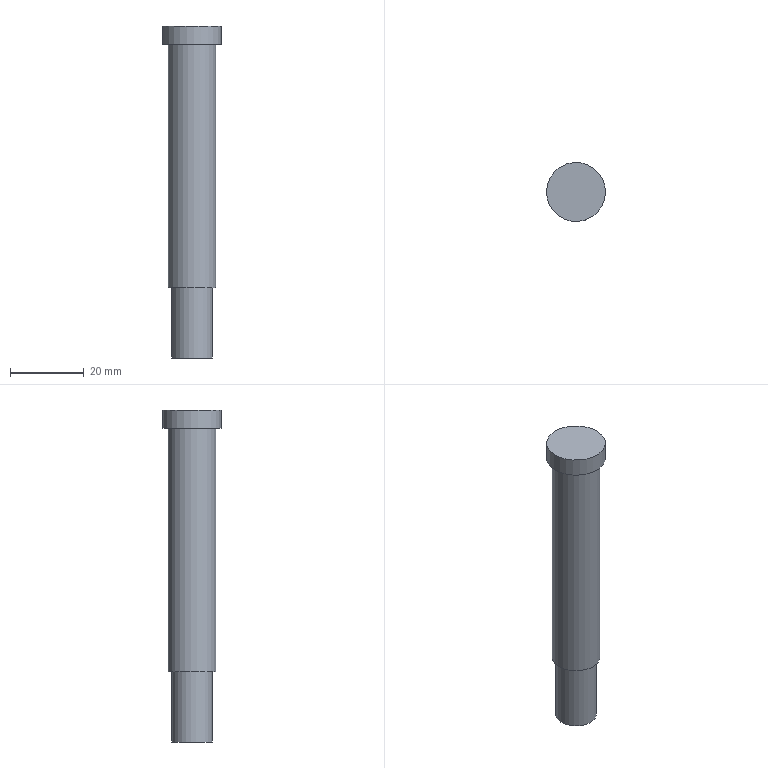Part | NX | features solid 2 | 1 solid | 7 faces | box 16 x 16 x 90 mm | volume 11604 mm3 | plane 4 | cylinder 3 | commonest cylinder face diameters 11.1 x1 13 x1 16 x1
STEP:
#1=CARTESIAN_POINT('',(-672.974,-368.75,22.));
#2=VERTEX_POINT('',#1);
#3=CARTESIAN_POINT('',(-678.603,-365.5,22.));
#4=DIRECTION('',(0.,0.,1.));
#5=DIRECTION('',(0.866,-0.5,0.));
#6=AXIS2_PLACEMENT_3D('',#3,#4,#5);
#7=CIRCLE('',#6,6.5);
#8=EDGE_CURVE('',#2,#2,#7,.T.);
#9=ORIENTED_EDGE('',*,*,#8,.T.);
#10=EDGE_LOOP('',(#9));
#11=FACE_BOUND('',#10,.T.);
#12=CARTESIAN_POINT('',(-672.974,-368.75,88.));
#13=VERTEX_POINT('',#12);
#14=CARTESIAN_POINT('',(-678.603,-365.5,88.));
#15=DIRECTION('',(0.,0.,1.));
#16=DIRECTION('',(0.866,-0.5,0.));
#17=AXIS2_PLACEMENT_3D('',#14,#15,#16);
#18=CIRCLE('',#17,6.5);
#19=EDGE_CURVE('',#13,#13,#18,.T.);
#20=ORIENTED_EDGE('',*,*,#19,.F.);
#21=EDGE_LOOP('',(#20));
#22=FACE_BOUND('',#21,.T.);
#23=CARTESIAN_POINT('',(-678.603,-365.5,93.));
#24=DIRECTION('',(0.,0.,-1.));
#25=DIRECTION('',(-0.866,0.5,0.));
#26=AXIS2_PLACEMENT_3D('',#23,#24,#25);
#27=CYLINDRICAL_SURFACE('',#26,6.5);
#28=ADVANCED_FACE('',(#11,#22),#27,.T.);
#29=CARTESIAN_POINT('',(-673.797,-368.275,22.));
#30=VERTEX_POINT('',#29);
#31=CARTESIAN_POINT('',(-678.603,-365.5,22.));
#32=DIRECTION('',(0.,0.,1.));
#33=DIRECTION('',(0.866,-0.5,0.));
#34=AXIS2_PLACEMENT_3D('',#31,#32,#33);
#35=CIRCLE('',#34,5.55);
#36=EDGE_CURVE('',#30,#30,#35,.T.);
#37=ORIENTED_EDGE('',*,*,#36,.T.);
#38=EDGE_LOOP('',(#37));
#39=FACE_BOUND('',#38,.T.);
#40=ORIENTED_EDGE('',*,*,#8,.F.);
#41=EDGE_LOOP('',(#40));
#42=FACE_BOUND('',#41,.T.);
#43=CARTESIAN_POINT('',(-678.603,-365.5,22.));
#44=DIRECTION('',(0.,0.,1.));
#45=DIRECTION('',(0.866,-0.5,0.));
#46=AXIS2_PLACEMENT_3D('',#43,#44,#45);
#47=PLANE('',#46);
#48=ADVANCED_FACE('',(#39,#42),#47,.F.);
#49=CARTESIAN_POINT('',(-671.675,-369.5,88.));
#50=VERTEX_POINT('',#49);
#51=CARTESIAN_POINT('',(-678.603,-365.5,88.));
#52=DIRECTION('',(0.,0.,1.));
#53=DIRECTION('',(0.866,-0.5,0.));
#54=AXIS2_PLACEMENT_3D('',#51,#52,#53);
#55=CIRCLE('',#54,8.);
#56=EDGE_CURVE('',#50,#50,#55,.T.);
#57=ORIENTED_EDGE('',*,*,#56,.F.);
#58=EDGE_LOOP('',(#57));
#59=FACE_BOUND('',#58,.T.);
#60=ORIENTED_EDGE('',*,*,#19,.T.);
#61=EDGE_LOOP('',(#60));
#62=FACE_BOUND('',#61,.T.);
#63=CARTESIAN_POINT('',(-678.603,-365.5,88.));
#64=DIRECTION('',(0.,0.,1.));
#65=DIRECTION('',(0.866,-0.5,0.));
#66=AXIS2_PLACEMENT_3D('',#63,#64,#65);
#67=PLANE('',#66);
#68=ADVANCED_FACE('',(#59,#62),#67,.F.);
#69=ORIENTED_EDGE('',*,*,#56,.T.);
#70=EDGE_LOOP('',(#69));
#71=FACE_BOUND('',#70,.T.);
#72=CARTESIAN_POINT('',(-671.675,-369.5,93.));
#73=VERTEX_POINT('',#72);
#74=CARTESIAN_POINT('',(-678.603,-365.5,93.));
#75=DIRECTION('',(0.,0.,1.));
#76=DIRECTION('',(0.866,-0.5,0.));
#77=AXIS2_PLACEMENT_3D('',#74,#75,#76);
#78=CIRCLE('',#77,8.);
#79=EDGE_CURVE('',#73,#73,#78,.T.);
#80=ORIENTED_EDGE('',*,*,#79,.F.);
#81=EDGE_LOOP('',(#80));
#82=FACE_BOUND('',#81,.T.);
#83=CARTESIAN_POINT('',(-678.603,-365.5,88.));
#84=DIRECTION('',(0.,0.,1.));
#85=DIRECTION('',(0.866,-0.5,0.));
#86=AXIS2_PLACEMENT_3D('',#83,#84,#85);
#87=CYLINDRICAL_SURFACE('',#86,8.);
#88=ADVANCED_FACE('',(#71,#82),#87,.T.);
#89=ORIENTED_EDGE('',*,*,#79,.T.);
#90=EDGE_LOOP('',(#89));
#91=FACE_BOUND('',#90,.T.);
#92=CARTESIAN_POINT('',(-678.603,-365.5,93.));
#93=DIRECTION('',(0.,0.,1.));
#94=DIRECTION('',(0.866,-0.5,0.));
#95=AXIS2_PLACEMENT_3D('',#92,#93,#94);
#96=PLANE('',#95);
#97=ADVANCED_FACE('',(#91),#96,.T.);
#98=CARTESIAN_POINT('',(-673.797,-368.275,3.));
#99=VERTEX_POINT('',#98);
#100=CARTESIAN_POINT('',(-678.603,-365.5,3.));
#101=DIRECTION('',(0.,0.,1.));
#102=DIRECTION('',(0.866,-0.5,0.));
#103=AXIS2_PLACEMENT_3D('',#100,#101,#102);
#104=CIRCLE('',#103,5.55);
#105=EDGE_CURVE('',#99,#99,#104,.T.);
#106=ORIENTED_EDGE('',*,*,#105,.T.);
#107=EDGE_LOOP('',(#106));
#108=FACE_BOUND('',#107,.T.);
#109=ORIENTED_EDGE('',*,*,#36,.F.);
#110=EDGE_LOOP('',(#109));
#111=FACE_BOUND('',#110,.T.);
#112=CARTESIAN_POINT('',(-678.603,-365.5,3.));
#113=DIRECTION('',(0.,0.,1.));
#114=DIRECTION('',(0.866,-0.5,0.));
#115=AXIS2_PLACEMENT_3D('',#112,#113,#114);
#116=CYLINDRICAL_SURFACE('',#115,5.55);
#117=ADVANCED_FACE('',(#108,#111),#116,.T.);
#118=ORIENTED_EDGE('',*,*,#105,.F.);
#119=EDGE_LOOP('',(#118));
#120=FACE_BOUND('',#119,.T.);
#121=CARTESIAN_POINT('',(-678.603,-365.5,3.));
#122=DIRECTION('',(0.,0.,1.));
#123=DIRECTION('',(0.866,-0.5,0.));
#124=AXIS2_PLACEMENT_3D('',#121,#122,#123);
#125=PLANE('',#124);
#126=ADVANCED_FACE('',(#120),#125,.F.);
#127=CLOSED_SHELL('',(#28,#48,#68,#88,#97,#117,#126));
#128=MANIFOLD_SOLID_BREP('',#127);
#129=(LENGTH_UNIT()NAMED_UNIT(*)SI_UNIT(.MILLI.,.METRE.));
#130=UNCERTAINTY_MEASURE_WITH_UNIT(LENGTH_MEASURE(0.00001),#129,'','');
#131=(NAMED_UNIT(*)PLANE_ANGLE_UNIT()SI_UNIT($,.RADIAN.));
#132=(NAMED_UNIT(*)SI_UNIT($,.STERADIAN.)SOLID_ANGLE_UNIT());
#133=(GEOMETRIC_REPRESENTATION_CONTEXT(3)GLOBAL_UNCERTAINTY_ASSIGNED_CONTEXT((#130))GLOBAL_UNIT_ASSIGNED_CONTEXT((#129,#131,#132))REPRESENTATION_CONTEXT('',''));
#134=ADVANCED_BREP_SHAPE_REPRESENTATION('',(#128),#133);